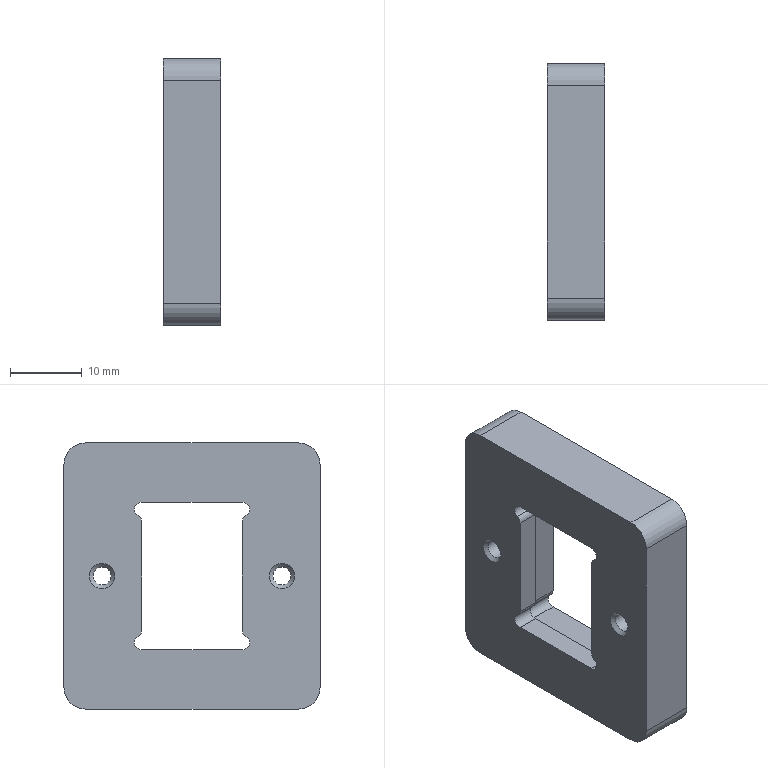Part | 1 solid | 41 faces | box 8 x 35.6 x 37 mm | volume 7524 mm3 | cylinder 22 | plane 15 | cone 4 | commonest cylinder face diameters 2 x16 6 x4 2.5 x2
STEP:
#1=CARTESIAN_POINT('',(288.112,-119.094,41.623));
#2=VERTEX_POINT('',#1);
#3=CARTESIAN_POINT('',(288.112,-122.094,38.623));
#4=VERTEX_POINT('',#3);
#5=CARTESIAN_POINT('',(288.112,-122.094,41.623));
#6=DIRECTION('',(-1.,0.,0.));
#7=DIRECTION('',(0.,-1.,0.));
#8=AXIS2_PLACEMENT_3D('',#5,#6,#7);
#9=CIRCLE('',#8,3.);
#10=EDGE_CURVE('',#2,#4,#9,.T.);
#11=ORIENTED_EDGE('',*,*,#10,.F.);
#12=CARTESIAN_POINT('',(296.112,-119.094,41.623));
#13=VERTEX_POINT('',#12);
#14=CARTESIAN_POINT('',(288.112,-119.094,41.623));
#15=DIRECTION('',(-1.,0.,0.));
#16=VECTOR('',#15,1000.);
#17=LINE('',#14,#16);
#18=EDGE_CURVE('',#13,#2,#17,.T.);
#19=ORIENTED_EDGE('',*,*,#18,.F.);
#20=CARTESIAN_POINT('',(296.112,-122.094,38.623));
#21=VERTEX_POINT('',#20);
#22=CARTESIAN_POINT('',(296.112,-122.094,41.623));
#23=DIRECTION('',(1.,0.,0.));
#24=DIRECTION('',(0.,-1.,0.));
#25=AXIS2_PLACEMENT_3D('',#22,#23,#24);
#26=CIRCLE('',#25,3.);
#27=EDGE_CURVE('',#21,#13,#26,.T.);
#28=ORIENTED_EDGE('',*,*,#27,.F.);
#29=CARTESIAN_POINT('',(288.112,-122.094,38.623));
#30=DIRECTION('',(1.,0.,0.));
#31=VECTOR('',#30,1000.);
#32=LINE('',#29,#31);
#33=EDGE_CURVE('',#4,#21,#32,.T.);
#34=ORIENTED_EDGE('',*,*,#33,.F.);
#35=EDGE_LOOP('',(#11,#19,#28,#34));
#36=FACE_BOUND('',#35,.T.);
#37=CARTESIAN_POINT('',(288.112,-122.094,41.623));
#38=DIRECTION('',(1.,0.,0.));
#39=DIRECTION('',(0.,-1.,0.));
#40=AXIS2_PLACEMENT_3D('',#37,#38,#39);
#41=CYLINDRICAL_SURFACE('',#40,3.);
#42=ADVANCED_FACE('',(#36),#41,.T.);
#43=CARTESIAN_POINT('',(288.112,-122.094,75.623));
#44=VERTEX_POINT('',#43);
#45=CARTESIAN_POINT('',(288.112,-119.094,72.623));
#46=VERTEX_POINT('',#45);
#47=CARTESIAN_POINT('',(288.112,-122.094,72.623));
#48=DIRECTION('',(-1.,0.,0.));
#49=DIRECTION('',(0.,-1.,0.));
#50=AXIS2_PLACEMENT_3D('',#47,#48,#49);
#51=CIRCLE('',#50,3.);
#52=EDGE_CURVE('',#44,#46,#51,.T.);
#53=ORIENTED_EDGE('',*,*,#52,.F.);
#54=CARTESIAN_POINT('',(296.112,-122.094,75.623));
#55=VERTEX_POINT('',#54);
#56=CARTESIAN_POINT('',(288.112,-122.094,75.623));
#57=DIRECTION('',(-1.,0.,0.));
#58=VECTOR('',#57,1000.);
#59=LINE('',#56,#58);
#60=EDGE_CURVE('',#55,#44,#59,.T.);
#61=ORIENTED_EDGE('',*,*,#60,.F.);
#62=CARTESIAN_POINT('',(296.112,-119.094,72.623));
#63=VERTEX_POINT('',#62);
#64=CARTESIAN_POINT('',(296.112,-122.094,72.623));
#65=DIRECTION('',(1.,0.,0.));
#66=DIRECTION('',(0.,-1.,0.));
#67=AXIS2_PLACEMENT_3D('',#64,#65,#66);
#68=CIRCLE('',#67,3.);
#69=EDGE_CURVE('',#63,#55,#68,.T.);
#70=ORIENTED_EDGE('',*,*,#69,.F.);
#71=CARTESIAN_POINT('',(288.112,-119.094,72.623));
#72=DIRECTION('',(1.,0.,0.));
#73=VECTOR('',#72,1000.);
#74=LINE('',#71,#73);
#75=EDGE_CURVE('',#46,#63,#74,.T.);
#76=ORIENTED_EDGE('',*,*,#75,.F.);
#77=EDGE_LOOP('',(#53,#61,#70,#76));
#78=FACE_BOUND('',#77,.T.);
#79=CARTESIAN_POINT('',(288.112,-122.094,72.623));
#80=DIRECTION('',(1.,0.,0.));
#81=DIRECTION('',(0.,-1.,0.));
#82=AXIS2_PLACEMENT_3D('',#79,#80,#81);
#83=CYLINDRICAL_SURFACE('',#82,3.);
#84=ADVANCED_FACE('',(#78),#83,.T.);
#85=CARTESIAN_POINT('',(288.112,-154.694,72.623));
#86=VERTEX_POINT('',#85);
#87=CARTESIAN_POINT('',(288.112,-151.694,75.623));
#88=VERTEX_POINT('',#87);
#89=CARTESIAN_POINT('',(288.112,-151.694,72.623));
#90=DIRECTION('',(-1.,0.,0.));
#91=DIRECTION('',(0.,-1.,0.));
#92=AXIS2_PLACEMENT_3D('',#89,#90,#91);
#93=CIRCLE('',#92,3.);
#94=EDGE_CURVE('',#86,#88,#93,.T.);
#95=ORIENTED_EDGE('',*,*,#94,.F.);
#96=CARTESIAN_POINT('',(296.112,-154.694,72.623));
#97=VERTEX_POINT('',#96);
#98=CARTESIAN_POINT('',(288.112,-154.694,72.623));
#99=DIRECTION('',(-1.,0.,0.));
#100=VECTOR('',#99,1000.);
#101=LINE('',#98,#100);
#102=EDGE_CURVE('',#97,#86,#101,.T.);
#103=ORIENTED_EDGE('',*,*,#102,.F.);
#104=CARTESIAN_POINT('',(296.112,-151.694,75.623));
#105=VERTEX_POINT('',#104);
#106=CARTESIAN_POINT('',(296.112,-151.694,72.623));
#107=DIRECTION('',(1.,0.,0.));
#108=DIRECTION('',(0.,-1.,0.));
#109=AXIS2_PLACEMENT_3D('',#106,#107,#108);
#110=CIRCLE('',#109,3.);
#111=EDGE_CURVE('',#105,#97,#110,.T.);
#112=ORIENTED_EDGE('',*,*,#111,.F.);
#113=CARTESIAN_POINT('',(288.112,-151.694,75.623));
#114=DIRECTION('',(1.,0.,0.));
#115=VECTOR('',#114,1000.);
#116=LINE('',#113,#115);
#117=EDGE_CURVE('',#88,#105,#116,.T.);
#118=ORIENTED_EDGE('',*,*,#117,.F.);
#119=EDGE_LOOP('',(#95,#103,#112,#118));
#120=FACE_BOUND('',#119,.T.);
#121=CARTESIAN_POINT('',(288.112,-151.694,72.623));
#122=DIRECTION('',(1.,0.,0.));
#123=DIRECTION('',(0.,-1.,0.));
#124=AXIS2_PLACEMENT_3D('',#121,#122,#123);
#125=CYLINDRICAL_SURFACE('',#124,3.);
#126=ADVANCED_FACE('',(#120),#125,.T.);
#127=CARTESIAN_POINT('',(288.112,-151.694,38.623));
#128=VERTEX_POINT('',#127);
#129=CARTESIAN_POINT('',(288.112,-154.694,41.623));
#130=VERTEX_POINT('',#129);
#131=CARTESIAN_POINT('',(288.112,-151.694,41.623));
#132=DIRECTION('',(-1.,0.,0.));
#133=DIRECTION('',(0.,-1.,0.));
#134=AXIS2_PLACEMENT_3D('',#131,#132,#133);
#135=CIRCLE('',#134,3.);
#136=EDGE_CURVE('',#128,#130,#135,.T.);
#137=ORIENTED_EDGE('',*,*,#136,.F.);
#138=CARTESIAN_POINT('',(296.112,-151.694,38.623));
#139=VERTEX_POINT('',#138);
#140=CARTESIAN_POINT('',(288.112,-151.694,38.623));
#141=DIRECTION('',(-1.,0.,0.));
#142=VECTOR('',#141,1000.);
#143=LINE('',#140,#142);
#144=EDGE_CURVE('',#139,#128,#143,.T.);
#145=ORIENTED_EDGE('',*,*,#144,.F.);
#146=CARTESIAN_POINT('',(296.112,-154.694,41.623));
#147=VERTEX_POINT('',#146);
#148=CARTESIAN_POINT('',(296.112,-151.694,41.623));
#149=DIRECTION('',(1.,0.,0.));
#150=DIRECTION('',(0.,-1.,0.));
#151=AXIS2_PLACEMENT_3D('',#148,#149,#150);
#152=CIRCLE('',#151,3.);
#153=EDGE_CURVE('',#147,#139,#152,.T.);
#154=ORIENTED_EDGE('',*,*,#153,.F.);
#155=CARTESIAN_POINT('',(288.112,-154.694,41.623));
#156=DIRECTION('',(1.,0.,0.));
#157=VECTOR('',#156,1000.);
#158=LINE('',#155,#157);
#159=EDGE_CURVE('',#130,#147,#158,.T.);
#160=ORIENTED_EDGE('',*,*,#159,.F.);
#161=EDGE_LOOP('',(#137,#145,#154,#160));
#162=FACE_BOUND('',#161,.T.);
#163=CARTESIAN_POINT('',(288.112,-151.694,41.623));
#164=DIRECTION('',(1.,0.,0.));
#165=DIRECTION('',(0.,-1.,0.));
#166=AXIS2_PLACEMENT_3D('',#163,#164,#165);
#167=CYLINDRICAL_SURFACE('',#166,3.);
#168=ADVANCED_FACE('',(#162),#167,.T.);
#169=CARTESIAN_POINT('',(291.112,-127.894,66.757));
#170=VERTEX_POINT('',#169);
#171=CARTESIAN_POINT('',(291.112,-128.394,68.623));
#172=VERTEX_POINT('',#171);
#173=CARTESIAN_POINT('',(291.112,-128.394,67.623));
#174=DIRECTION('',(1.,0.,0.));
#175=DIRECTION('',(0.,-1.,0.));
#176=AXIS2_PLACEMENT_3D('',#173,#174,#175);
#177=CIRCLE('',#176,1.);
#178=EDGE_CURVE('',#170,#172,#177,.T.);
#179=ORIENTED_EDGE('',*,*,#178,.F.);
#180=CARTESIAN_POINT('',(296.112,-127.894,66.757));
#181=VERTEX_POINT('',#180);
#182=CARTESIAN_POINT('',(296.112,-127.894,66.757));
#183=DIRECTION('',(1.,0.,0.));
#184=VECTOR('',#183,1000.);
#185=LINE('',#182,#184);
#186=EDGE_CURVE('',#170,#181,#185,.T.);
#187=ORIENTED_EDGE('',*,*,#186,.T.);
#188=CARTESIAN_POINT('',(296.112,-128.394,68.623));
#189=VERTEX_POINT('',#188);
#190=CARTESIAN_POINT('',(296.112,-128.394,67.623));
#191=DIRECTION('',(1.,0.,0.));
#192=DIRECTION('',(0.,-1.,0.));
#193=AXIS2_PLACEMENT_3D('',#190,#191,#192);
#194=CIRCLE('',#193,1.);
#195=EDGE_CURVE('',#181,#189,#194,.T.);
#196=ORIENTED_EDGE('',*,*,#195,.T.);
#197=CARTESIAN_POINT('',(291.112,-128.394,68.623));
#198=DIRECTION('',(1.,0.,0.));
#199=VECTOR('',#198,1000.);
#200=LINE('',#197,#199);
#201=EDGE_CURVE('',#172,#189,#200,.T.);
#202=ORIENTED_EDGE('',*,*,#201,.F.);
#203=EDGE_LOOP('',(#179,#187,#196,#202));
#204=FACE_BOUND('',#203,.T.);
#205=CARTESIAN_POINT('',(296.112,-128.394,67.623));
#206=DIRECTION('',(1.,0.,0.));
#207=DIRECTION('',(0.,-1.,0.));
#208=AXIS2_PLACEMENT_3D('',#205,#206,#207);
#209=CYLINDRICAL_SURFACE('',#208,1.);
#210=ADVANCED_FACE('',(#204),#209,.F.);
#211=CARTESIAN_POINT('',(296.112,-128.394,45.623));
#212=VERTEX_POINT('',#211);
#213=CARTESIAN_POINT('',(296.112,-127.894,47.489));
#214=VERTEX_POINT('',#213);
#215=CARTESIAN_POINT('',(296.112,-128.394,46.623));
#216=DIRECTION('',(1.,0.,0.));
#217=DIRECTION('',(0.,-1.,0.));
#218=AXIS2_PLACEMENT_3D('',#215,#216,#217);
#219=CIRCLE('',#218,1.);
#220=EDGE_CURVE('',#212,#214,#219,.T.);
#221=ORIENTED_EDGE('',*,*,#220,.T.);
#222=CARTESIAN_POINT('',(291.112,-127.894,47.489));
#223=VERTEX_POINT('',#222);
#224=CARTESIAN_POINT('',(296.112,-127.894,47.489));
#225=DIRECTION('',(1.,0.,0.));
#226=VECTOR('',#225,1000.);
#227=LINE('',#224,#226);
#228=EDGE_CURVE('',#214,#223,#227,.F.);
#229=ORIENTED_EDGE('',*,*,#228,.T.);
#230=CARTESIAN_POINT('',(291.112,-128.394,45.623));
#231=VERTEX_POINT('',#230);
#232=CARTESIAN_POINT('',(291.112,-128.394,46.623));
#233=DIRECTION('',(1.,0.,0.));
#234=DIRECTION('',(0.,-1.,0.));
#235=AXIS2_PLACEMENT_3D('',#232,#233,#234);
#236=CIRCLE('',#235,1.);
#237=EDGE_CURVE('',#231,#223,#236,.T.);
#238=ORIENTED_EDGE('',*,*,#237,.F.);
#239=CARTESIAN_POINT('',(291.112,-128.394,45.623));
#240=DIRECTION('',(1.,0.,0.));
#241=VECTOR('',#240,1000.);
#242=LINE('',#239,#241);
#243=EDGE_CURVE('',#231,#212,#242,.T.);
#244=ORIENTED_EDGE('',*,*,#243,.T.);
#245=EDGE_LOOP('',(#221,#229,#238,#244));
#246=FACE_BOUND('',#245,.T.);
#247=CARTESIAN_POINT('',(296.112,-128.394,46.623));
#248=DIRECTION('',(1.,0.,0.));
#249=DIRECTION('',(0.,-1.,0.));
#250=AXIS2_PLACEMENT_3D('',#247,#248,#249);
#251=CYLINDRICAL_SURFACE('',#250,1.);
#252=ADVANCED_FACE('',(#246),#251,.F.);
#253=CARTESIAN_POINT('',(288.112,-129.394,65.507));
#254=VERTEX_POINT('',#253);
#255=CARTESIAN_POINT('',(288.112,-129.894,67.373));
#256=VERTEX_POINT('',#255);
#257=CARTESIAN_POINT('',(288.112,-129.894,66.373));
#258=DIRECTION('',(1.,0.,0.));
#259=DIRECTION('',(0.,-1.,0.));
#260=AXIS2_PLACEMENT_3D('',#257,#258,#259);
#261=CIRCLE('',#260,1.);
#262=EDGE_CURVE('',#254,#256,#261,.T.);
#263=ORIENTED_EDGE('',*,*,#262,.F.);
#264=CARTESIAN_POINT('',(291.112,-129.394,65.507));
#265=VERTEX_POINT('',#264);
#266=CARTESIAN_POINT('',(288.112,-129.394,65.507));
#267=DIRECTION('',(1.,0.,0.));
#268=VECTOR('',#267,1000.);
#269=LINE('',#266,#268);
#270=EDGE_CURVE('',#254,#265,#269,.T.);
#271=ORIENTED_EDGE('',*,*,#270,.T.);
#272=CARTESIAN_POINT('',(291.112,-129.894,67.373));
#273=VERTEX_POINT('',#272);
#274=CARTESIAN_POINT('',(291.112,-129.894,66.373));
#275=DIRECTION('',(1.,0.,0.));
#276=DIRECTION('',(0.,-1.,0.));
#277=AXIS2_PLACEMENT_3D('',#274,#275,#276);
#278=CIRCLE('',#277,1.);
#279=EDGE_CURVE('',#265,#273,#278,.T.);
#280=ORIENTED_EDGE('',*,*,#279,.T.);
#281=CARTESIAN_POINT('',(288.112,-129.894,67.373));
#282=DIRECTION('',(1.,0.,0.));
#283=VECTOR('',#282,1000.);
#284=LINE('',#281,#283);
#285=EDGE_CURVE('',#256,#273,#284,.T.);
#286=ORIENTED_EDGE('',*,*,#285,.F.);
#287=EDGE_LOOP('',(#263,#271,#280,#286));
#288=FACE_BOUND('',#287,.T.);
#289=CARTESIAN_POINT('',(288.112,-129.894,66.373));
#290=DIRECTION('',(1.,0.,0.));
#291=DIRECTION('',(0.,-1.,0.));
#292=AXIS2_PLACEMENT_3D('',#289,#290,#291);
#293=CYLINDRICAL_SURFACE('',#292,1.);
#294=ADVANCED_FACE('',(#288),#293,.F.);
#295=CARTESIAN_POINT('',(291.112,-129.894,46.873));
#296=VERTEX_POINT('',#295);
#297=CARTESIAN_POINT('',(291.112,-129.394,48.739));
#298=VERTEX_POINT('',#297);
#299=CARTESIAN_POINT('',(291.112,-129.894,47.873));
#300=DIRECTION('',(1.,0.,0.));
#301=DIRECTION('',(0.,-1.,0.));
#302=AXIS2_PLACEMENT_3D('',#299,#300,#301);
#303=CIRCLE('',#302,1.);
#304=EDGE_CURVE('',#296,#298,#303,.T.);
#305=ORIENTED_EDGE('',*,*,#304,.T.);
#306=CARTESIAN_POINT('',(288.112,-129.394,48.739));
#307=VERTEX_POINT('',#306);
#308=CARTESIAN_POINT('',(288.112,-129.394,48.739));
#309=DIRECTION('',(1.,0.,0.));
#310=VECTOR('',#309,1000.);
#311=LINE('',#308,#310);
#312=EDGE_CURVE('',#298,#307,#311,.F.);
#313=ORIENTED_EDGE('',*,*,#312,.T.);
#314=CARTESIAN_POINT('',(288.112,-129.894,46.873));
#315=VERTEX_POINT('',#314);
#316=CARTESIAN_POINT('',(288.112,-129.894,47.873));
#317=DIRECTION('',(1.,0.,0.));
#318=DIRECTION('',(0.,-1.,0.));
#319=AXIS2_PLACEMENT_3D('',#316,#317,#318);
#320=CIRCLE('',#319,1.);
#321=EDGE_CURVE('',#315,#307,#320,.T.);
#322=ORIENTED_EDGE('',*,*,#321,.F.);
#323=CARTESIAN_POINT('',(288.112,-129.894,46.873));
#324=DIRECTION('',(1.,0.,0.));
#325=VECTOR('',#324,1000.);
#326=LINE('',#323,#325);
#327=EDGE_CURVE('',#315,#296,#326,.T.);
#328=ORIENTED_EDGE('',*,*,#327,.T.);
#329=EDGE_LOOP('',(#305,#313,#322,#328));
#330=FACE_BOUND('',#329,.T.);
#331=CARTESIAN_POINT('',(288.112,-129.894,47.873));
#332=DIRECTION('',(1.,0.,0.));
#333=DIRECTION('',(0.,-1.,0.));
#334=AXIS2_PLACEMENT_3D('',#331,#332,#333);
#335=CYLINDRICAL_SURFACE('',#334,1.);
#336=ADVANCED_FACE('',(#330),#335,.F.);
#337=CARTESIAN_POINT('',(296.112,-145.394,45.623));
#338=VERTEX_POINT('',#337);
#339=CARTESIAN_POINT('',(296.112,-128.394,45.623));
#340=DIRECTION('',(0.,1.,0.));
#341=VECTOR('',#340,1000.);
#342=LINE('',#339,#341);
#343=EDGE_CURVE('',#338,#212,#342,.T.);
#344=ORIENTED_EDGE('',*,*,#343,.T.);
#345=ORIENTED_EDGE('',*,*,#243,.F.);
#346=CARTESIAN_POINT('',(291.112,-145.394,45.623));
#347=VERTEX_POINT('',#346);
#348=CARTESIAN_POINT('',(291.112,-128.394,45.623));
#349=DIRECTION('',(0.,1.,0.));
#350=VECTOR('',#349,1000.);
#351=LINE('',#348,#350);
#352=EDGE_CURVE('',#347,#231,#351,.T.);
#353=ORIENTED_EDGE('',*,*,#352,.F.);
#354=CARTESIAN_POINT('',(291.112,-145.394,45.623));
#355=DIRECTION('',(1.,0.,0.));
#356=VECTOR('',#355,1000.);
#357=LINE('',#354,#356);
#358=EDGE_CURVE('',#347,#338,#357,.T.);
#359=ORIENTED_EDGE('',*,*,#358,.T.);
#360=EDGE_LOOP('',(#344,#345,#353,#359));
#361=FACE_BOUND('',#360,.T.);
#362=CARTESIAN_POINT('',(291.112,-128.394,45.623));
#363=DIRECTION('',(0.,0.,-1.));
#364=DIRECTION('',(-1.,0.,0.));
#365=AXIS2_PLACEMENT_3D('',#362,#363,#364);
#366=PLANE('',#365);
#367=ADVANCED_FACE('',(#361),#366,.F.);
#368=CARTESIAN_POINT('',(296.112,-145.394,68.623));
#369=VERTEX_POINT('',#368);
#370=CARTESIAN_POINT('',(296.112,-128.394,68.623));
#371=DIRECTION('',(0.,-1.,0.));
#372=VECTOR('',#371,1000.);
#373=LINE('',#370,#372);
#374=EDGE_CURVE('',#189,#369,#373,.T.);
#375=ORIENTED_EDGE('',*,*,#374,.T.);
#376=CARTESIAN_POINT('',(291.112,-145.394,68.623));
#377=VERTEX_POINT('',#376);
#378=CARTESIAN_POINT('',(291.112,-145.394,68.623));
#379=DIRECTION('',(1.,0.,0.));
#380=VECTOR('',#379,1000.);
#381=LINE('',#378,#380);
#382=EDGE_CURVE('',#377,#369,#381,.T.);
#383=ORIENTED_EDGE('',*,*,#382,.F.);
#384=CARTESIAN_POINT('',(291.112,-128.394,68.623));
#385=DIRECTION('',(0.,-1.,0.));
#386=VECTOR('',#385,1000.);
#387=LINE('',#384,#386);
#388=EDGE_CURVE('',#172,#377,#387,.T.);
#389=ORIENTED_EDGE('',*,*,#388,.F.);
#390=ORIENTED_EDGE('',*,*,#201,.T.);
#391=EDGE_LOOP('',(#375,#383,#389,#390));
#392=FACE_BOUND('',#391,.T.);
#393=CARTESIAN_POINT('',(291.112,-128.394,68.623));
#394=DIRECTION('',(0.,0.,1.));
#395=DIRECTION('',(0.,-1.,0.));
#396=AXIS2_PLACEMENT_3D('',#393,#394,#395);
#397=PLANE('',#396);
#398=ADVANCED_FACE('',(#392),#397,.F.);
#399=ORIENTED_EDGE('',*,*,#388,.T.);
#400=CARTESIAN_POINT('',(291.112,-145.894,66.757));
#401=VERTEX_POINT('',#400);
#402=CARTESIAN_POINT('',(291.112,-145.394,67.623));
#403=DIRECTION('',(1.,0.,0.));
#404=DIRECTION('',(0.,-1.,0.));
#405=AXIS2_PLACEMENT_3D('',#402,#403,#404);
#406=CIRCLE('',#405,1.);
#407=EDGE_CURVE('',#377,#401,#406,.T.);
#408=ORIENTED_EDGE('',*,*,#407,.T.);
#409=CARTESIAN_POINT('',(291.112,-145.394,65.891));
#410=VERTEX_POINT('',#409);
#411=CARTESIAN_POINT('',(291.112,-146.394,65.891));
#412=DIRECTION('',(1.,0.,0.));
#413=DIRECTION('',(0.,0.,-1.));
#414=AXIS2_PLACEMENT_3D('',#411,#412,#413);
#415=CIRCLE('',#414,1.);
#416=EDGE_CURVE('',#401,#410,#415,.F.);
#417=ORIENTED_EDGE('',*,*,#416,.T.);
#418=CARTESIAN_POINT('',(291.112,-145.394,48.355));
#419=VERTEX_POINT('',#418);
#420=CARTESIAN_POINT('',(291.112,-145.394,45.623));
#421=DIRECTION('',(0.,0.,-1.));
#422=VECTOR('',#421,1000.);
#423=LINE('',#420,#422);
#424=EDGE_CURVE('',#410,#419,#423,.T.);
#425=ORIENTED_EDGE('',*,*,#424,.T.);
#426=CARTESIAN_POINT('',(291.112,-145.894,47.489));
#427=VERTEX_POINT('',#426);
#428=CARTESIAN_POINT('',(291.112,-146.394,48.355));
#429=DIRECTION('',(1.,0.,0.));
#430=DIRECTION('',(0.,0.,-1.));
#431=AXIS2_PLACEMENT_3D('',#428,#429,#430);
#432=CIRCLE('',#431,1.);
#433=EDGE_CURVE('',#419,#427,#432,.F.);
#434=ORIENTED_EDGE('',*,*,#433,.T.);
#435=CARTESIAN_POINT('',(291.112,-145.394,46.623));
#436=DIRECTION('',(1.,0.,0.));
#437=DIRECTION('',(0.,-1.,0.));
#438=AXIS2_PLACEMENT_3D('',#435,#436,#437);
#439=CIRCLE('',#438,1.);
#440=EDGE_CURVE('',#427,#347,#439,.T.);
#441=ORIENTED_EDGE('',*,*,#440,.T.);
#442=ORIENTED_EDGE('',*,*,#352,.T.);
#443=ORIENTED_EDGE('',*,*,#237,.T.);
#444=CARTESIAN_POINT('',(291.112,-128.394,48.355));
#445=VERTEX_POINT('',#444);
#446=CARTESIAN_POINT('',(291.112,-127.394,48.355));
#447=DIRECTION('',(1.,0.,0.));
#448=DIRECTION('',(0.,0.,-1.));
#449=AXIS2_PLACEMENT_3D('',#446,#447,#448);
#450=CIRCLE('',#449,1.);
#451=EDGE_CURVE('',#223,#445,#450,.F.);
#452=ORIENTED_EDGE('',*,*,#451,.T.);
#453=CARTESIAN_POINT('',(291.112,-128.394,65.891));
#454=VERTEX_POINT('',#453);
#455=CARTESIAN_POINT('',(291.112,-128.394,45.623));
#456=DIRECTION('',(0.,0.,1.));
#457=VECTOR('',#456,1000.);
#458=LINE('',#455,#457);
#459=EDGE_CURVE('',#445,#454,#458,.T.);
#460=ORIENTED_EDGE('',*,*,#459,.T.);
#461=CARTESIAN_POINT('',(291.112,-127.394,65.891));
#462=DIRECTION('',(1.,0.,0.));
#463=DIRECTION('',(0.,0.,-1.));
#464=AXIS2_PLACEMENT_3D('',#461,#462,#463);
#465=CIRCLE('',#464,1.);
#466=EDGE_CURVE('',#454,#170,#465,.F.);
#467=ORIENTED_EDGE('',*,*,#466,.T.);
#468=ORIENTED_EDGE('',*,*,#178,.T.);
#469=EDGE_LOOP('',(#399,#408,#417,#425,#434,#441,#442,#443,#452,#460,#467,#468));
#470=FACE_BOUND('',#469,.T.);
#471=CARTESIAN_POINT('',(291.112,-129.894,64.641));
#472=VERTEX_POINT('',#471);
#473=CARTESIAN_POINT('',(291.112,-129.894,49.605));
#474=VERTEX_POINT('',#473);
#475=CARTESIAN_POINT('',(291.112,-129.894,46.873));
#476=DIRECTION('',(0.,0.,-1.));
#477=VECTOR('',#476,1000.);
#478=LINE('',#475,#477);
#479=EDGE_CURVE('',#472,#474,#478,.T.);
#480=ORIENTED_EDGE('',*,*,#479,.T.);
#481=CARTESIAN_POINT('',(291.112,-128.894,49.605));
#482=DIRECTION('',(1.,0.,0.));
#483=DIRECTION('',(0.,0.,-1.));
#484=AXIS2_PLACEMENT_3D('',#481,#482,#483);
#485=CIRCLE('',#484,1.);
#486=EDGE_CURVE('',#474,#298,#485,.T.);
#487=ORIENTED_EDGE('',*,*,#486,.T.);
#488=ORIENTED_EDGE('',*,*,#304,.F.);
#489=CARTESIAN_POINT('',(291.112,-143.894,46.873));
#490=VERTEX_POINT('',#489);
#491=CARTESIAN_POINT('',(291.112,-129.894,46.873));
#492=DIRECTION('',(0.,-1.,0.));
#493=VECTOR('',#492,1000.);
#494=LINE('',#491,#493);
#495=EDGE_CURVE('',#296,#490,#494,.T.);
#496=ORIENTED_EDGE('',*,*,#495,.T.);
#497=CARTESIAN_POINT('',(291.112,-144.394,48.739));
#498=VERTEX_POINT('',#497);
#499=CARTESIAN_POINT('',(291.112,-143.894,47.873));
#500=DIRECTION('',(1.,0.,0.));
#501=DIRECTION('',(0.,-1.,0.));
#502=AXIS2_PLACEMENT_3D('',#499,#500,#501);
#503=CIRCLE('',#502,1.);
#504=EDGE_CURVE('',#498,#490,#503,.T.);
#505=ORIENTED_EDGE('',*,*,#504,.F.);
#506=CARTESIAN_POINT('',(291.112,-143.894,49.605));
#507=VERTEX_POINT('',#506);
#508=CARTESIAN_POINT('',(291.112,-144.894,49.605));
#509=DIRECTION('',(1.,0.,0.));
#510=DIRECTION('',(0.,0.,-1.));
#511=AXIS2_PLACEMENT_3D('',#508,#509,#510);
#512=CIRCLE('',#511,1.);
#513=EDGE_CURVE('',#498,#507,#512,.T.);
#514=ORIENTED_EDGE('',*,*,#513,.T.);
#515=CARTESIAN_POINT('',(291.112,-143.894,64.641));
#516=VERTEX_POINT('',#515);
#517=CARTESIAN_POINT('',(291.112,-143.894,46.873));
#518=DIRECTION('',(0.,0.,1.));
#519=VECTOR('',#518,1000.);
#520=LINE('',#517,#519);
#521=EDGE_CURVE('',#507,#516,#520,.T.);
#522=ORIENTED_EDGE('',*,*,#521,.T.);
#523=CARTESIAN_POINT('',(291.112,-144.394,65.507));
#524=VERTEX_POINT('',#523);
#525=CARTESIAN_POINT('',(291.112,-144.894,64.641));
#526=DIRECTION('',(1.,0.,0.));
#527=DIRECTION('',(0.,0.,-1.));
#528=AXIS2_PLACEMENT_3D('',#525,#526,#527);
#529=CIRCLE('',#528,1.);
#530=EDGE_CURVE('',#516,#524,#529,.T.);
#531=ORIENTED_EDGE('',*,*,#530,.T.);
#532=CARTESIAN_POINT('',(291.112,-143.894,67.373));
#533=VERTEX_POINT('',#532);
#534=CARTESIAN_POINT('',(291.112,-143.894,66.373));
#535=DIRECTION('',(1.,0.,0.));
#536=DIRECTION('',(0.,-1.,0.));
#537=AXIS2_PLACEMENT_3D('',#534,#535,#536);
#538=CIRCLE('',#537,1.);
#539=EDGE_CURVE('',#533,#524,#538,.T.);
#540=ORIENTED_EDGE('',*,*,#539,.F.);
#541=CARTESIAN_POINT('',(291.112,-129.894,67.373));
#542=DIRECTION('',(0.,1.,0.));
#543=VECTOR('',#542,1000.);
#544=LINE('',#541,#543);
#545=EDGE_CURVE('',#533,#273,#544,.T.);
#546=ORIENTED_EDGE('',*,*,#545,.T.);
#547=ORIENTED_EDGE('',*,*,#279,.F.);
#548=CARTESIAN_POINT('',(291.112,-128.894,64.641));
#549=DIRECTION('',(1.,0.,0.));
#550=DIRECTION('',(0.,0.,-1.));
#551=AXIS2_PLACEMENT_3D('',#548,#549,#550);
#552=CIRCLE('',#551,1.);
#553=EDGE_CURVE('',#265,#472,#552,.T.);
#554=ORIENTED_EDGE('',*,*,#553,.T.);
#555=EDGE_LOOP('',(#480,#487,#488,#496,#505,#514,#522,#531,#540,#546,#547,#554));
#556=FACE_BOUND('',#555,.T.);
#557=CARTESIAN_POINT('',(291.112,-136.894,57.123));
#558=DIRECTION('',(1.,0.,0.));
#559=DIRECTION('',(0.,0.,1.));
#560=AXIS2_PLACEMENT_3D('',#557,#558,#559);
#561=PLANE('',#560);
#562=ADVANCED_FACE('',(#470,#556),#561,.T.);
#563=CARTESIAN_POINT('',(296.112,-154.694,38.623));
#564=DIRECTION('',(0.,0.,-1.));
#565=VECTOR('',#564,1000.);
#566=LINE('',#563,#565);
#567=EDGE_CURVE('',#97,#147,#566,.T.);
#568=ORIENTED_EDGE('',*,*,#567,.T.);
#569=ORIENTED_EDGE('',*,*,#153,.T.);
#570=CARTESIAN_POINT('',(296.112,-119.094,38.623));
#571=DIRECTION('',(0.,1.,0.));
#572=VECTOR('',#571,1000.);
#573=LINE('',#570,#572);
#574=EDGE_CURVE('',#139,#21,#573,.T.);
#575=ORIENTED_EDGE('',*,*,#574,.T.);
#576=ORIENTED_EDGE('',*,*,#27,.T.);
#577=CARTESIAN_POINT('',(296.112,-119.094,38.623));
#578=DIRECTION('',(0.,0.,1.));
#579=VECTOR('',#578,1000.);
#580=LINE('',#577,#579);
#581=EDGE_CURVE('',#13,#63,#580,.T.);
#582=ORIENTED_EDGE('',*,*,#581,.T.);
#583=ORIENTED_EDGE('',*,*,#69,.T.);
#584=CARTESIAN_POINT('',(296.112,-119.094,75.623));
#585=DIRECTION('',(0.,-1.,0.));
#586=VECTOR('',#585,1000.);
#587=LINE('',#584,#586);
#588=EDGE_CURVE('',#55,#105,#587,.T.);
#589=ORIENTED_EDGE('',*,*,#588,.T.);
#590=ORIENTED_EDGE('',*,*,#111,.T.);
#591=EDGE_LOOP('',(#568,#569,#575,#576,#582,#583,#589,#590));
#592=FACE_BOUND('',#591,.T.);
#593=CARTESIAN_POINT('',(296.112,-128.394,48.355));
#594=VERTEX_POINT('',#593);
#595=CARTESIAN_POINT('',(296.112,-128.394,65.891));
#596=VERTEX_POINT('',#595);
#597=CARTESIAN_POINT('',(296.112,-128.394,45.623));
#598=DIRECTION('',(0.,0.,1.));
#599=VECTOR('',#598,1000.);
#600=LINE('',#597,#599);
#601=EDGE_CURVE('',#594,#596,#600,.T.);
#602=ORIENTED_EDGE('',*,*,#601,.F.);
#603=CARTESIAN_POINT('',(296.112,-127.394,48.355));
#604=DIRECTION('',(1.,0.,0.));
#605=DIRECTION('',(0.,0.,-1.));
#606=AXIS2_PLACEMENT_3D('',#603,#604,#605);
#607=CIRCLE('',#606,1.);
#608=EDGE_CURVE('',#594,#214,#607,.T.);
#609=ORIENTED_EDGE('',*,*,#608,.T.);
#610=ORIENTED_EDGE('',*,*,#220,.F.);
#611=ORIENTED_EDGE('',*,*,#343,.F.);
#612=CARTESIAN_POINT('',(296.112,-145.894,47.489));
#613=VERTEX_POINT('',#612);
#614=CARTESIAN_POINT('',(296.112,-145.394,46.623));
#615=DIRECTION('',(1.,0.,0.));
#616=DIRECTION('',(0.,-1.,0.));
#617=AXIS2_PLACEMENT_3D('',#614,#615,#616);
#618=CIRCLE('',#617,1.);
#619=EDGE_CURVE('',#613,#338,#618,.T.);
#620=ORIENTED_EDGE('',*,*,#619,.F.);
#621=CARTESIAN_POINT('',(296.112,-145.394,48.355));
#622=VERTEX_POINT('',#621);
#623=CARTESIAN_POINT('',(296.112,-146.394,48.355));
#624=DIRECTION('',(1.,0.,0.));
#625=DIRECTION('',(0.,0.,-1.));
#626=AXIS2_PLACEMENT_3D('',#623,#624,#625);
#627=CIRCLE('',#626,1.);
#628=EDGE_CURVE('',#613,#622,#627,.T.);
#629=ORIENTED_EDGE('',*,*,#628,.T.);
#630=CARTESIAN_POINT('',(296.112,-145.394,65.891));
#631=VERTEX_POINT('',#630);
#632=CARTESIAN_POINT('',(296.112,-145.394,45.623));
#633=DIRECTION('',(0.,0.,-1.));
#634=VECTOR('',#633,1000.);
#635=LINE('',#632,#634);
#636=EDGE_CURVE('',#631,#622,#635,.T.);
#637=ORIENTED_EDGE('',*,*,#636,.F.);
#638=CARTESIAN_POINT('',(296.112,-145.894,66.757));
#639=VERTEX_POINT('',#638);
#640=CARTESIAN_POINT('',(296.112,-146.394,65.891));
#641=DIRECTION('',(1.,0.,0.));
#642=DIRECTION('',(0.,0.,-1.));
#643=AXIS2_PLACEMENT_3D('',#640,#641,#642);
#644=CIRCLE('',#643,1.);
#645=EDGE_CURVE('',#631,#639,#644,.T.);
#646=ORIENTED_EDGE('',*,*,#645,.T.);
#647=CARTESIAN_POINT('',(296.112,-145.394,67.623));
#648=DIRECTION('',(1.,0.,0.));
#649=DIRECTION('',(0.,-1.,0.));
#650=AXIS2_PLACEMENT_3D('',#647,#648,#649);
#651=CIRCLE('',#650,1.);
#652=EDGE_CURVE('',#369,#639,#651,.T.);
#653=ORIENTED_EDGE('',*,*,#652,.F.);
#654=ORIENTED_EDGE('',*,*,#374,.F.);
#655=ORIENTED_EDGE('',*,*,#195,.F.);
#656=CARTESIAN_POINT('',(296.112,-127.394,65.891));
#657=DIRECTION('',(1.,0.,0.));
#658=DIRECTION('',(0.,0.,-1.));
#659=AXIS2_PLACEMENT_3D('',#656,#657,#658);
#660=CIRCLE('',#659,1.);
#661=EDGE_CURVE('',#181,#596,#660,.T.);
#662=ORIENTED_EDGE('',*,*,#661,.T.);
#663=EDGE_LOOP('',(#602,#609,#610,#611,#620,#629,#637,#646,#653,#654,#655,#662));
#664=FACE_BOUND('',#663,.T.);
#665=CARTESIAN_POINT('',(296.112,-126.144,57.123));
#666=VERTEX_POINT('',#665);
#667=CARTESIAN_POINT('',(296.112,-124.394,57.123));
#668=DIRECTION('',(-1.,0.,0.));
#669=DIRECTION('',(0.,-1.,0.));
#670=AXIS2_PLACEMENT_3D('',#667,#668,#669);
#671=CIRCLE('',#670,1.75);
#672=EDGE_CURVE('',#666,#666,#671,.T.);
#673=ORIENTED_EDGE('',*,*,#672,.T.);
#674=EDGE_LOOP('',(#673));
#675=FACE_BOUND('',#674,.T.);
#676=CARTESIAN_POINT('',(296.112,-151.144,57.123));
#677=VERTEX_POINT('',#676);
#678=CARTESIAN_POINT('',(296.112,-149.394,57.123));
#679=DIRECTION('',(-1.,0.,0.));
#680=DIRECTION('',(0.,-1.,0.));
#681=AXIS2_PLACEMENT_3D('',#678,#679,#680);
#682=CIRCLE('',#681,1.75);
#683=EDGE_CURVE('',#677,#677,#682,.T.);
#684=ORIENTED_EDGE('',*,*,#683,.T.);
#685=EDGE_LOOP('',(#684));
#686=FACE_BOUND('',#685,.T.);
#687=CARTESIAN_POINT('',(296.112,-136.894,57.123));
#688=DIRECTION('',(1.,0.,0.));
#689=DIRECTION('',(0.,0.,1.));
#690=AXIS2_PLACEMENT_3D('',#687,#688,#689);
#691=PLANE('',#690);
#692=ADVANCED_FACE('',(#592,#664,#675,#686),#691,.T.);
#693=CARTESIAN_POINT('',(288.112,-119.094,38.623));
#694=DIRECTION('',(0.,1.,0.));
#695=VECTOR('',#694,1000.);
#696=LINE('',#693,#695);
#697=EDGE_CURVE('',#128,#4,#696,.T.);
#698=ORIENTED_EDGE('',*,*,#697,.F.);
#699=ORIENTED_EDGE('',*,*,#136,.T.);
#700=CARTESIAN_POINT('',(288.112,-154.694,38.623));
#701=DIRECTION('',(0.,0.,-1.));
#702=VECTOR('',#701,1000.);
#703=LINE('',#700,#702);
#704=EDGE_CURVE('',#86,#130,#703,.T.);
#705=ORIENTED_EDGE('',*,*,#704,.F.);
#706=ORIENTED_EDGE('',*,*,#94,.T.);
#707=CARTESIAN_POINT('',(288.112,-119.094,75.623));
#708=DIRECTION('',(0.,-1.,0.));
#709=VECTOR('',#708,1000.);
#710=LINE('',#707,#709);
#711=EDGE_CURVE('',#44,#88,#710,.T.);
#712=ORIENTED_EDGE('',*,*,#711,.F.);
#713=ORIENTED_EDGE('',*,*,#52,.T.);
#714=CARTESIAN_POINT('',(288.112,-119.094,38.623));
#715=DIRECTION('',(0.,0.,1.));
#716=VECTOR('',#715,1000.);
#717=LINE('',#714,#716);
#718=EDGE_CURVE('',#2,#46,#717,.T.);
#719=ORIENTED_EDGE('',*,*,#718,.F.);
#720=ORIENTED_EDGE('',*,*,#10,.T.);
#721=EDGE_LOOP('',(#698,#699,#705,#706,#712,#713,#719,#720));
#722=FACE_BOUND('',#721,.T.);
#723=ORIENTED_EDGE('',*,*,#321,.T.);
#724=CARTESIAN_POINT('',(288.112,-129.894,49.605));
#725=VERTEX_POINT('',#724);
#726=CARTESIAN_POINT('',(288.112,-128.894,49.605));
#727=DIRECTION('',(1.,0.,0.));
#728=DIRECTION('',(0.,0.,-1.));
#729=AXIS2_PLACEMENT_3D('',#726,#727,#728);
#730=CIRCLE('',#729,1.);
#731=EDGE_CURVE('',#307,#725,#730,.F.);
#732=ORIENTED_EDGE('',*,*,#731,.T.);
#733=CARTESIAN_POINT('',(288.112,-129.894,64.641));
#734=VERTEX_POINT('',#733);
#735=CARTESIAN_POINT('',(288.112,-129.894,46.873));
#736=DIRECTION('',(0.,0.,1.));
#737=VECTOR('',#736,1000.);
#738=LINE('',#735,#737);
#739=EDGE_CURVE('',#725,#734,#738,.T.);
#740=ORIENTED_EDGE('',*,*,#739,.T.);
#741=CARTESIAN_POINT('',(288.112,-128.894,64.641));
#742=DIRECTION('',(1.,0.,0.));
#743=DIRECTION('',(0.,0.,-1.));
#744=AXIS2_PLACEMENT_3D('',#741,#742,#743);
#745=CIRCLE('',#744,1.);
#746=EDGE_CURVE('',#734,#254,#745,.F.);
#747=ORIENTED_EDGE('',*,*,#746,.T.);
#748=ORIENTED_EDGE('',*,*,#262,.T.);
#749=CARTESIAN_POINT('',(288.112,-143.894,67.373));
#750=VERTEX_POINT('',#749);
#751=CARTESIAN_POINT('',(288.112,-129.894,67.373));
#752=DIRECTION('',(0.,-1.,0.));
#753=VECTOR('',#752,1000.);
#754=LINE('',#751,#753);
#755=EDGE_CURVE('',#256,#750,#754,.T.);
#756=ORIENTED_EDGE('',*,*,#755,.T.);
#757=CARTESIAN_POINT('',(288.112,-144.394,65.507));
#758=VERTEX_POINT('',#757);
#759=CARTESIAN_POINT('',(288.112,-143.894,66.373));
#760=DIRECTION('',(1.,0.,0.));
#761=DIRECTION('',(0.,-1.,0.));
#762=AXIS2_PLACEMENT_3D('',#759,#760,#761);
#763=CIRCLE('',#762,1.);
#764=EDGE_CURVE('',#750,#758,#763,.T.);
#765=ORIENTED_EDGE('',*,*,#764,.T.);
#766=CARTESIAN_POINT('',(288.112,-143.894,64.641));
#767=VERTEX_POINT('',#766);
#768=CARTESIAN_POINT('',(288.112,-144.894,64.641));
#769=DIRECTION('',(1.,0.,0.));
#770=DIRECTION('',(0.,0.,-1.));
#771=AXIS2_PLACEMENT_3D('',#768,#769,#770);
#772=CIRCLE('',#771,1.);
#773=EDGE_CURVE('',#758,#767,#772,.F.);
#774=ORIENTED_EDGE('',*,*,#773,.T.);
#775=CARTESIAN_POINT('',(288.112,-143.894,49.605));
#776=VERTEX_POINT('',#775);
#777=CARTESIAN_POINT('',(288.112,-143.894,46.873));
#778=DIRECTION('',(0.,0.,-1.));
#779=VECTOR('',#778,1000.);
#780=LINE('',#777,#779);
#781=EDGE_CURVE('',#767,#776,#780,.T.);
#782=ORIENTED_EDGE('',*,*,#781,.T.);
#783=CARTESIAN_POINT('',(288.112,-144.394,48.739));
#784=VERTEX_POINT('',#783);
#785=CARTESIAN_POINT('',(288.112,-144.894,49.605));
#786=DIRECTION('',(1.,0.,0.));
#787=DIRECTION('',(0.,0.,-1.));
#788=AXIS2_PLACEMENT_3D('',#785,#786,#787);
#789=CIRCLE('',#788,1.);
#790=EDGE_CURVE('',#776,#784,#789,.F.);
#791=ORIENTED_EDGE('',*,*,#790,.T.);
#792=CARTESIAN_POINT('',(288.112,-143.894,46.873));
#793=VERTEX_POINT('',#792);
#794=CARTESIAN_POINT('',(288.112,-143.894,47.873));
#795=DIRECTION('',(1.,0.,0.));
#796=DIRECTION('',(0.,-1.,0.));
#797=AXIS2_PLACEMENT_3D('',#794,#795,#796);
#798=CIRCLE('',#797,1.);
#799=EDGE_CURVE('',#784,#793,#798,.T.);
#800=ORIENTED_EDGE('',*,*,#799,.T.);
#801=CARTESIAN_POINT('',(288.112,-129.894,46.873));
#802=DIRECTION('',(0.,1.,0.));
#803=VECTOR('',#802,1000.);
#804=LINE('',#801,#803);
#805=EDGE_CURVE('',#793,#315,#804,.T.);
#806=ORIENTED_EDGE('',*,*,#805,.T.);
#807=EDGE_LOOP('',(#723,#732,#740,#747,#748,#756,#765,#774,#782,#791,#800,#806));
#808=FACE_BOUND('',#807,.T.);
#809=CARTESIAN_POINT('',(288.112,-126.144,57.123));
#810=VERTEX_POINT('',#809);
#811=CARTESIAN_POINT('',(288.112,-124.394,57.123));
#812=DIRECTION('',(1.,0.,0.));
#813=DIRECTION('',(0.,-1.,0.));
#814=AXIS2_PLACEMENT_3D('',#811,#812,#813);
#815=CIRCLE('',#814,1.75);
#816=EDGE_CURVE('',#810,#810,#815,.T.);
#817=ORIENTED_EDGE('',*,*,#816,.T.);
#818=EDGE_LOOP('',(#817));
#819=FACE_BOUND('',#818,.T.);
#820=CARTESIAN_POINT('',(288.112,-151.144,57.123));
#821=VERTEX_POINT('',#820);
#822=CARTESIAN_POINT('',(288.112,-149.394,57.123));
#823=DIRECTION('',(1.,0.,0.));
#824=DIRECTION('',(0.,-1.,0.));
#825=AXIS2_PLACEMENT_3D('',#822,#823,#824);
#826=CIRCLE('',#825,1.75);
#827=EDGE_CURVE('',#821,#821,#826,.T.);
#828=ORIENTED_EDGE('',*,*,#827,.T.);
#829=EDGE_LOOP('',(#828));
#830=FACE_BOUND('',#829,.T.);
#831=CARTESIAN_POINT('',(288.112,-136.894,57.123));
#832=DIRECTION('',(1.,0.,0.));
#833=DIRECTION('',(0.,0.,1.));
#834=AXIS2_PLACEMENT_3D('',#831,#832,#833);
#835=PLANE('',#834);
#836=ADVANCED_FACE('',(#722,#808,#819,#830),#835,.F.);
#837=ORIENTED_EDGE('',*,*,#574,.F.);
#838=ORIENTED_EDGE('',*,*,#144,.T.);
#839=ORIENTED_EDGE('',*,*,#697,.T.);
#840=ORIENTED_EDGE('',*,*,#33,.T.);
#841=EDGE_LOOP('',(#837,#838,#839,#840));
#842=FACE_BOUND('',#841,.T.);
#843=CARTESIAN_POINT('',(288.112,-119.094,38.623));
#844=DIRECTION('',(0.,0.,-1.));
#845=DIRECTION('',(-1.,0.,0.));
#846=AXIS2_PLACEMENT_3D('',#843,#844,#845);
#847=PLANE('',#846);
#848=ADVANCED_FACE('',(#842),#847,.T.);
#849=ORIENTED_EDGE('',*,*,#718,.T.);
#850=ORIENTED_EDGE('',*,*,#75,.T.);
#851=ORIENTED_EDGE('',*,*,#581,.F.);
#852=ORIENTED_EDGE('',*,*,#18,.T.);
#853=EDGE_LOOP('',(#849,#850,#851,#852));
#854=FACE_BOUND('',#853,.T.);
#855=CARTESIAN_POINT('',(288.112,-119.094,38.623));
#856=DIRECTION('',(0.,1.,0.));
#857=DIRECTION('',(0.,0.,-1.));
#858=AXIS2_PLACEMENT_3D('',#855,#856,#857);
#859=PLANE('',#858);
#860=ADVANCED_FACE('',(#854),#859,.T.);
#861=ORIENTED_EDGE('',*,*,#711,.T.);
#862=ORIENTED_EDGE('',*,*,#117,.T.);
#863=ORIENTED_EDGE('',*,*,#588,.F.);
#864=ORIENTED_EDGE('',*,*,#60,.T.);
#865=EDGE_LOOP('',(#861,#862,#863,#864));
#866=FACE_BOUND('',#865,.T.);
#867=CARTESIAN_POINT('',(288.112,-119.094,75.623));
#868=DIRECTION('',(0.,0.,1.));
#869=DIRECTION('',(0.,-1.,0.));
#870=AXIS2_PLACEMENT_3D('',#867,#868,#869);
#871=PLANE('',#870);
#872=ADVANCED_FACE('',(#866),#871,.T.);
#873=ORIENTED_EDGE('',*,*,#704,.T.);
#874=ORIENTED_EDGE('',*,*,#159,.T.);
#875=ORIENTED_EDGE('',*,*,#567,.F.);
#876=ORIENTED_EDGE('',*,*,#102,.T.);
#877=EDGE_LOOP('',(#873,#874,#875,#876));
#878=FACE_BOUND('',#877,.T.);
#879=CARTESIAN_POINT('',(288.112,-154.694,38.623));
#880=DIRECTION('',(0.,-1.,0.));
#881=DIRECTION('',(0.,0.,-1.));
#882=AXIS2_PLACEMENT_3D('',#879,#880,#881);
#883=PLANE('',#882);
#884=ADVANCED_FACE('',(#878),#883,.T.);
#885=ORIENTED_EDGE('',*,*,#495,.F.);
#886=ORIENTED_EDGE('',*,*,#327,.F.);
#887=ORIENTED_EDGE('',*,*,#805,.F.);
#888=CARTESIAN_POINT('',(288.112,-143.894,46.873));
#889=DIRECTION('',(1.,0.,0.));
#890=VECTOR('',#889,1000.);
#891=LINE('',#888,#890);
#892=EDGE_CURVE('',#793,#490,#891,.T.);
#893=ORIENTED_EDGE('',*,*,#892,.T.);
#894=EDGE_LOOP('',(#885,#886,#887,#893));
#895=FACE_BOUND('',#894,.T.);
#896=CARTESIAN_POINT('',(288.112,-129.894,46.873));
#897=DIRECTION('',(0.,0.,-1.));
#898=DIRECTION('',(-1.,0.,0.));
#899=AXIS2_PLACEMENT_3D('',#896,#897,#898);
#900=PLANE('',#899);
#901=ADVANCED_FACE('',(#895),#900,.F.);
#902=ORIENTED_EDGE('',*,*,#739,.F.);
#903=CARTESIAN_POINT('',(288.112,-129.894,49.605));
#904=DIRECTION('',(1.,0.,0.));
#905=VECTOR('',#904,1000.);
#906=LINE('',#903,#905);
#907=EDGE_CURVE('',#725,#474,#906,.T.);
#908=ORIENTED_EDGE('',*,*,#907,.T.);
#909=ORIENTED_EDGE('',*,*,#479,.F.);
#910=CARTESIAN_POINT('',(288.112,-129.894,64.641));
#911=DIRECTION('',(1.,0.,0.));
#912=VECTOR('',#911,1000.);
#913=LINE('',#910,#912);
#914=EDGE_CURVE('',#472,#734,#913,.F.);
#915=ORIENTED_EDGE('',*,*,#914,.T.);
#916=EDGE_LOOP('',(#902,#908,#909,#915));
#917=FACE_BOUND('',#916,.T.);
#918=CARTESIAN_POINT('',(288.112,-129.894,46.873));
#919=DIRECTION('',(0.,1.,0.));
#920=DIRECTION('',(0.,0.,-1.));
#921=AXIS2_PLACEMENT_3D('',#918,#919,#920);
#922=PLANE('',#921);
#923=ADVANCED_FACE('',(#917),#922,.F.);
#924=ORIENTED_EDGE('',*,*,#545,.F.);
#925=CARTESIAN_POINT('',(288.112,-143.894,67.373));
#926=DIRECTION('',(1.,0.,0.));
#927=VECTOR('',#926,1000.);
#928=LINE('',#925,#927);
#929=EDGE_CURVE('',#750,#533,#928,.T.);
#930=ORIENTED_EDGE('',*,*,#929,.F.);
#931=ORIENTED_EDGE('',*,*,#755,.F.);
#932=ORIENTED_EDGE('',*,*,#285,.T.);
#933=EDGE_LOOP('',(#924,#930,#931,#932));
#934=FACE_BOUND('',#933,.T.);
#935=CARTESIAN_POINT('',(288.112,-129.894,67.373));
#936=DIRECTION('',(0.,0.,1.));
#937=DIRECTION('',(0.,-1.,0.));
#938=AXIS2_PLACEMENT_3D('',#935,#936,#937);
#939=PLANE('',#938);
#940=ADVANCED_FACE('',(#934),#939,.F.);
#941=ORIENTED_EDGE('',*,*,#521,.F.);
#942=CARTESIAN_POINT('',(288.112,-143.894,49.605));
#943=DIRECTION('',(1.,0.,0.));
#944=VECTOR('',#943,1000.);
#945=LINE('',#942,#944);
#946=EDGE_CURVE('',#507,#776,#945,.F.);
#947=ORIENTED_EDGE('',*,*,#946,.T.);
#948=ORIENTED_EDGE('',*,*,#781,.F.);
#949=CARTESIAN_POINT('',(288.112,-143.894,64.641));
#950=DIRECTION('',(1.,0.,0.));
#951=VECTOR('',#950,1000.);
#952=LINE('',#949,#951);
#953=EDGE_CURVE('',#767,#516,#952,.T.);
#954=ORIENTED_EDGE('',*,*,#953,.T.);
#955=EDGE_LOOP('',(#941,#947,#948,#954));
#956=FACE_BOUND('',#955,.T.);
#957=CARTESIAN_POINT('',(288.112,-143.894,46.873));
#958=DIRECTION('',(0.,-1.,0.));
#959=DIRECTION('',(0.,0.,-1.));
#960=AXIS2_PLACEMENT_3D('',#957,#958,#959);
#961=PLANE('',#960);
#962=ADVANCED_FACE('',(#956),#961,.F.);
#963=ORIENTED_EDGE('',*,*,#459,.F.);
#964=CARTESIAN_POINT('',(291.112,-128.394,48.355));
#965=DIRECTION('',(1.,0.,0.));
#966=VECTOR('',#965,1000.);
#967=LINE('',#964,#966);
#968=EDGE_CURVE('',#445,#594,#967,.T.);
#969=ORIENTED_EDGE('',*,*,#968,.T.);
#970=ORIENTED_EDGE('',*,*,#601,.T.);
#971=CARTESIAN_POINT('',(291.112,-128.394,65.891));
#972=DIRECTION('',(1.,0.,0.));
#973=VECTOR('',#972,1000.);
#974=LINE('',#971,#973);
#975=EDGE_CURVE('',#596,#454,#974,.F.);
#976=ORIENTED_EDGE('',*,*,#975,.T.);
#977=EDGE_LOOP('',(#963,#969,#970,#976));
#978=FACE_BOUND('',#977,.T.);
#979=CARTESIAN_POINT('',(291.112,-128.394,45.623));
#980=DIRECTION('',(0.,1.,0.));
#981=DIRECTION('',(0.,0.,-1.));
#982=AXIS2_PLACEMENT_3D('',#979,#980,#981);
#983=PLANE('',#982);
#984=ADVANCED_FACE('',(#978),#983,.F.);
#985=ORIENTED_EDGE('',*,*,#636,.T.);
#986=CARTESIAN_POINT('',(291.112,-145.394,48.355));
#987=DIRECTION('',(1.,0.,0.));
#988=VECTOR('',#987,1000.);
#989=LINE('',#986,#988);
#990=EDGE_CURVE('',#622,#419,#989,.F.);
#991=ORIENTED_EDGE('',*,*,#990,.T.);
#992=ORIENTED_EDGE('',*,*,#424,.F.);
#993=CARTESIAN_POINT('',(291.112,-145.394,65.891));
#994=DIRECTION('',(1.,0.,0.));
#995=VECTOR('',#994,1000.);
#996=LINE('',#993,#995);
#997=EDGE_CURVE('',#410,#631,#996,.T.);
#998=ORIENTED_EDGE('',*,*,#997,.T.);
#999=EDGE_LOOP('',(#985,#991,#992,#998));
#1000=FACE_BOUND('',#999,.T.);
#1001=CARTESIAN_POINT('',(291.112,-145.394,45.623));
#1002=DIRECTION('',(0.,-1.,0.));
#1003=DIRECTION('',(0.,0.,-1.));
#1004=AXIS2_PLACEMENT_3D('',#1001,#1002,#1003);
#1005=PLANE('',#1004);
#1006=ADVANCED_FACE('',(#1000),#1005,.F.);
#1007=ORIENTED_EDGE('',*,*,#539,.T.);
#1008=CARTESIAN_POINT('',(288.112,-144.394,65.507));
#1009=DIRECTION('',(1.,0.,0.));
#1010=VECTOR('',#1009,1000.);
#1011=LINE('',#1008,#1010);
#1012=EDGE_CURVE('',#524,#758,#1011,.F.);
#1013=ORIENTED_EDGE('',*,*,#1012,.T.);
#1014=ORIENTED_EDGE('',*,*,#764,.F.);
#1015=ORIENTED_EDGE('',*,*,#929,.T.);
#1016=EDGE_LOOP('',(#1007,#1013,#1014,#1015));
#1017=FACE_BOUND('',#1016,.T.);
#1018=CARTESIAN_POINT('',(288.112,-143.894,66.373));
#1019=DIRECTION('',(1.,0.,0.));
#1020=DIRECTION('',(0.,-1.,0.));
#1021=AXIS2_PLACEMENT_3D('',#1018,#1019,#1020);
#1022=CYLINDRICAL_SURFACE('',#1021,1.);
#1023=ADVANCED_FACE('',(#1017),#1022,.F.);
#1024=ORIENTED_EDGE('',*,*,#799,.F.);
#1025=CARTESIAN_POINT('',(288.112,-144.394,48.739));
#1026=DIRECTION('',(1.,0.,0.));
#1027=VECTOR('',#1026,1000.);
#1028=LINE('',#1025,#1027);
#1029=EDGE_CURVE('',#784,#498,#1028,.T.);
#1030=ORIENTED_EDGE('',*,*,#1029,.T.);
#1031=ORIENTED_EDGE('',*,*,#504,.T.);
#1032=ORIENTED_EDGE('',*,*,#892,.F.);
#1033=EDGE_LOOP('',(#1024,#1030,#1031,#1032));
#1034=FACE_BOUND('',#1033,.T.);
#1035=CARTESIAN_POINT('',(288.112,-143.894,47.873));
#1036=DIRECTION('',(1.,0.,0.));
#1037=DIRECTION('',(0.,-1.,0.));
#1038=AXIS2_PLACEMENT_3D('',#1035,#1036,#1037);
#1039=CYLINDRICAL_SURFACE('',#1038,1.);
#1040=ADVANCED_FACE('',(#1034),#1039,.F.);
#1041=ORIENTED_EDGE('',*,*,#440,.F.);
#1042=CARTESIAN_POINT('',(296.112,-145.894,47.489));
#1043=DIRECTION('',(1.,0.,0.));
#1044=VECTOR('',#1043,1000.);
#1045=LINE('',#1042,#1044);
#1046=EDGE_CURVE('',#427,#613,#1045,.T.);
#1047=ORIENTED_EDGE('',*,*,#1046,.T.);
#1048=ORIENTED_EDGE('',*,*,#619,.T.);
#1049=ORIENTED_EDGE('',*,*,#358,.F.);
#1050=EDGE_LOOP('',(#1041,#1047,#1048,#1049));
#1051=FACE_BOUND('',#1050,.T.);
#1052=CARTESIAN_POINT('',(296.112,-145.394,46.623));
#1053=DIRECTION('',(1.,0.,0.));
#1054=DIRECTION('',(0.,-1.,0.));
#1055=AXIS2_PLACEMENT_3D('',#1052,#1053,#1054);
#1056=CYLINDRICAL_SURFACE('',#1055,1.);
#1057=ADVANCED_FACE('',(#1051),#1056,.F.);
#1058=ORIENTED_EDGE('',*,*,#652,.T.);
#1059=CARTESIAN_POINT('',(296.112,-145.894,66.757));
#1060=DIRECTION('',(1.,0.,0.));
#1061=VECTOR('',#1060,1000.);
#1062=LINE('',#1059,#1061);
#1063=EDGE_CURVE('',#639,#401,#1062,.F.);
#1064=ORIENTED_EDGE('',*,*,#1063,.T.);
#1065=ORIENTED_EDGE('',*,*,#407,.F.);
#1066=ORIENTED_EDGE('',*,*,#382,.T.);
#1067=EDGE_LOOP('',(#1058,#1064,#1065,#1066));
#1068=FACE_BOUND('',#1067,.T.);
#1069=CARTESIAN_POINT('',(296.112,-145.394,67.623));
#1070=DIRECTION('',(1.,0.,0.));
#1071=DIRECTION('',(0.,-1.,0.));
#1072=AXIS2_PLACEMENT_3D('',#1069,#1070,#1071);
#1073=CYLINDRICAL_SURFACE('',#1072,1.);
#1074=ADVANCED_FACE('',(#1068),#1073,.F.);
#1075=CARTESIAN_POINT('',(295.612,-150.644,57.123));
#1076=VERTEX_POINT('',#1075);
#1077=CARTESIAN_POINT('',(295.612,-149.394,57.123));
#1078=DIRECTION('',(1.,0.,0.));
#1079=DIRECTION('',(0.,-1.,0.));
#1080=AXIS2_PLACEMENT_3D('',#1077,#1078,#1079);
#1081=CIRCLE('',#1080,1.25);
#1082=EDGE_CURVE('',#1076,#1076,#1081,.T.);
#1083=ORIENTED_EDGE('',*,*,#1082,.T.);
#1084=EDGE_LOOP('',(#1083));
#1085=FACE_BOUND('',#1084,.T.);
#1086=CARTESIAN_POINT('',(288.612,-150.644,57.123));
#1087=VERTEX_POINT('',#1086);
#1088=CARTESIAN_POINT('',(288.612,-149.394,57.123));
#1089=DIRECTION('',(-1.,0.,0.));
#1090=DIRECTION('',(0.,-1.,0.));
#1091=AXIS2_PLACEMENT_3D('',#1088,#1089,#1090);
#1092=CIRCLE('',#1091,1.25);
#1093=EDGE_CURVE('',#1087,#1087,#1092,.T.);
#1094=ORIENTED_EDGE('',*,*,#1093,.T.);
#1095=EDGE_LOOP('',(#1094));
#1096=FACE_BOUND('',#1095,.T.);
#1097=CARTESIAN_POINT('',(296.112,-149.394,57.123));
#1098=DIRECTION('',(1.,0.,0.));
#1099=DIRECTION('',(0.,-1.,0.));
#1100=AXIS2_PLACEMENT_3D('',#1097,#1098,#1099);
#1101=CYLINDRICAL_SURFACE('',#1100,1.25);
#1102=ADVANCED_FACE('',(#1085,#1096),#1101,.F.);
#1103=CARTESIAN_POINT('',(295.612,-125.644,57.123));
#1104=VERTEX_POINT('',#1103);
#1105=CARTESIAN_POINT('',(295.612,-124.394,57.123));
#1106=DIRECTION('',(1.,0.,0.));
#1107=DIRECTION('',(0.,-1.,0.));
#1108=AXIS2_PLACEMENT_3D('',#1105,#1106,#1107);
#1109=CIRCLE('',#1108,1.25);
#1110=EDGE_CURVE('',#1104,#1104,#1109,.T.);
#1111=ORIENTED_EDGE('',*,*,#1110,.T.);
#1112=EDGE_LOOP('',(#1111));
#1113=FACE_BOUND('',#1112,.T.);
#1114=CARTESIAN_POINT('',(288.612,-125.644,57.123));
#1115=VERTEX_POINT('',#1114);
#1116=CARTESIAN_POINT('',(288.612,-124.394,57.123));
#1117=DIRECTION('',(-1.,0.,0.));
#1118=DIRECTION('',(0.,-1.,0.));
#1119=AXIS2_PLACEMENT_3D('',#1116,#1117,#1118);
#1120=CIRCLE('',#1119,1.25);
#1121=EDGE_CURVE('',#1115,#1115,#1120,.T.);
#1122=ORIENTED_EDGE('',*,*,#1121,.T.);
#1123=EDGE_LOOP('',(#1122));
#1124=FACE_BOUND('',#1123,.T.);
#1125=CARTESIAN_POINT('',(296.112,-124.394,57.123));
#1126=DIRECTION('',(1.,0.,0.));
#1127=DIRECTION('',(0.,-1.,0.));
#1128=AXIS2_PLACEMENT_3D('',#1125,#1126,#1127);
#1129=CYLINDRICAL_SURFACE('',#1128,1.25);
#1130=ADVANCED_FACE('',(#1113,#1124),#1129,.F.);
#1131=ORIENTED_EDGE('',*,*,#1093,.F.);
#1132=EDGE_LOOP('',(#1131));
#1133=FACE_BOUND('',#1132,.T.);
#1134=ORIENTED_EDGE('',*,*,#827,.F.);
#1135=EDGE_LOOP('',(#1134));
#1136=FACE_BOUND('',#1135,.T.);
#1137=CARTESIAN_POINT('',(288.112,-149.394,57.123));
#1138=DIRECTION('',(-1.,0.,0.));
#1139=DIRECTION('',(0.,1.,0.));
#1140=AXIS2_PLACEMENT_3D('',#1137,#1138,#1139);
#1141=CONICAL_SURFACE('',#1140,1.75,0.7854);
#1142=ADVANCED_FACE('',(#1133,#1136),#1141,.F.);
#1143=ORIENTED_EDGE('',*,*,#683,.F.);
#1144=EDGE_LOOP('',(#1143));
#1145=FACE_BOUND('',#1144,.T.);
#1146=ORIENTED_EDGE('',*,*,#1082,.F.);
#1147=EDGE_LOOP('',(#1146));
#1148=FACE_BOUND('',#1147,.T.);
#1149=CARTESIAN_POINT('',(295.612,-149.394,57.123));
#1150=DIRECTION('',(1.,0.,0.));
#1151=DIRECTION('',(0.,-1.,0.));
#1152=AXIS2_PLACEMENT_3D('',#1149,#1150,#1151);
#1153=CONICAL_SURFACE('',#1152,1.25,0.7854);
#1154=ADVANCED_FACE('',(#1145,#1148),#1153,.F.);
#1155=ORIENTED_EDGE('',*,*,#1121,.F.);
#1156=EDGE_LOOP('',(#1155));
#1157=FACE_BOUND('',#1156,.T.);
#1158=ORIENTED_EDGE('',*,*,#816,.F.);
#1159=EDGE_LOOP('',(#1158));
#1160=FACE_BOUND('',#1159,.T.);
#1161=CARTESIAN_POINT('',(288.112,-124.394,57.123));
#1162=DIRECTION('',(-1.,0.,0.));
#1163=DIRECTION('',(0.,1.,0.));
#1164=AXIS2_PLACEMENT_3D('',#1161,#1162,#1163);
#1165=CONICAL_SURFACE('',#1164,1.75,0.7854);
#1166=ADVANCED_FACE('',(#1157,#1160),#1165,.F.);
#1167=ORIENTED_EDGE('',*,*,#672,.F.);
#1168=EDGE_LOOP('',(#1167));
#1169=FACE_BOUND('',#1168,.T.);
#1170=ORIENTED_EDGE('',*,*,#1110,.F.);
#1171=EDGE_LOOP('',(#1170));
#1172=FACE_BOUND('',#1171,.T.);
#1173=CARTESIAN_POINT('',(295.612,-124.394,57.123));
#1174=DIRECTION('',(1.,0.,0.));
#1175=DIRECTION('',(0.,-1.,0.));
#1176=AXIS2_PLACEMENT_3D('',#1173,#1174,#1175);
#1177=CONICAL_SURFACE('',#1176,1.25,0.7854);
#1178=ADVANCED_FACE('',(#1169,#1172),#1177,.F.);
#1179=ORIENTED_EDGE('',*,*,#731,.F.);
#1180=ORIENTED_EDGE('',*,*,#312,.F.);
#1181=ORIENTED_EDGE('',*,*,#486,.F.);
#1182=ORIENTED_EDGE('',*,*,#907,.F.);
#1183=EDGE_LOOP('',(#1179,#1180,#1181,#1182));
#1184=FACE_BOUND('',#1183,.T.);
#1185=CARTESIAN_POINT('',(288.112,-128.894,49.605));
#1186=DIRECTION('',(1.,0.,0.));
#1187=DIRECTION('',(0.,0.,-1.));
#1188=AXIS2_PLACEMENT_3D('',#1185,#1186,#1187);
#1189=CYLINDRICAL_SURFACE('',#1188,1.);
#1190=ADVANCED_FACE('',(#1184),#1189,.T.);
#1191=ORIENTED_EDGE('',*,*,#608,.F.);
#1192=ORIENTED_EDGE('',*,*,#968,.F.);
#1193=ORIENTED_EDGE('',*,*,#451,.F.);
#1194=ORIENTED_EDGE('',*,*,#228,.F.);
#1195=EDGE_LOOP('',(#1191,#1192,#1193,#1194));
#1196=FACE_BOUND('',#1195,.T.);
#1197=CARTESIAN_POINT('',(296.112,-127.394,48.355));
#1198=DIRECTION('',(1.,0.,0.));
#1199=DIRECTION('',(0.,0.,-1.));
#1200=AXIS2_PLACEMENT_3D('',#1197,#1198,#1199);
#1201=CYLINDRICAL_SURFACE('',#1200,1.);
#1202=ADVANCED_FACE('',(#1196),#1201,.T.);
#1203=ORIENTED_EDGE('',*,*,#553,.F.);
#1204=ORIENTED_EDGE('',*,*,#270,.F.);
#1205=ORIENTED_EDGE('',*,*,#746,.F.);
#1206=ORIENTED_EDGE('',*,*,#914,.F.);
#1207=EDGE_LOOP('',(#1203,#1204,#1205,#1206));
#1208=FACE_BOUND('',#1207,.T.);
#1209=CARTESIAN_POINT('',(288.112,-128.894,64.641));
#1210=DIRECTION('',(1.,0.,0.));
#1211=DIRECTION('',(0.,0.,-1.));
#1212=AXIS2_PLACEMENT_3D('',#1209,#1210,#1211);
#1213=CYLINDRICAL_SURFACE('',#1212,1.);
#1214=ADVANCED_FACE('',(#1208),#1213,.T.);
#1215=ORIENTED_EDGE('',*,*,#661,.F.);
#1216=ORIENTED_EDGE('',*,*,#186,.F.);
#1217=ORIENTED_EDGE('',*,*,#466,.F.);
#1218=ORIENTED_EDGE('',*,*,#975,.F.);
#1219=EDGE_LOOP('',(#1215,#1216,#1217,#1218));
#1220=FACE_BOUND('',#1219,.T.);
#1221=CARTESIAN_POINT('',(296.112,-127.394,65.891));
#1222=DIRECTION('',(1.,0.,0.));
#1223=DIRECTION('',(0.,0.,-1.));
#1224=AXIS2_PLACEMENT_3D('',#1221,#1222,#1223);
#1225=CYLINDRICAL_SURFACE('',#1224,1.);
#1226=ADVANCED_FACE('',(#1220),#1225,.T.);
#1227=ORIENTED_EDGE('',*,*,#628,.F.);
#1228=ORIENTED_EDGE('',*,*,#1046,.F.);
#1229=ORIENTED_EDGE('',*,*,#433,.F.);
#1230=ORIENTED_EDGE('',*,*,#990,.F.);
#1231=EDGE_LOOP('',(#1227,#1228,#1229,#1230));
#1232=FACE_BOUND('',#1231,.T.);
#1233=CARTESIAN_POINT('',(296.112,-146.394,48.355));
#1234=DIRECTION('',(1.,0.,0.));
#1235=DIRECTION('',(0.,0.,-1.));
#1236=AXIS2_PLACEMENT_3D('',#1233,#1234,#1235);
#1237=CYLINDRICAL_SURFACE('',#1236,1.);
#1238=ADVANCED_FACE('',(#1232),#1237,.T.);
#1239=ORIENTED_EDGE('',*,*,#513,.F.);
#1240=ORIENTED_EDGE('',*,*,#1029,.F.);
#1241=ORIENTED_EDGE('',*,*,#790,.F.);
#1242=ORIENTED_EDGE('',*,*,#946,.F.);
#1243=EDGE_LOOP('',(#1239,#1240,#1241,#1242));
#1244=FACE_BOUND('',#1243,.T.);
#1245=CARTESIAN_POINT('',(288.112,-144.894,49.605));
#1246=DIRECTION('',(1.,0.,0.));
#1247=DIRECTION('',(0.,0.,-1.));
#1248=AXIS2_PLACEMENT_3D('',#1245,#1246,#1247);
#1249=CYLINDRICAL_SURFACE('',#1248,1.);
#1250=ADVANCED_FACE('',(#1244),#1249,.T.);
#1251=ORIENTED_EDGE('',*,*,#645,.F.);
#1252=ORIENTED_EDGE('',*,*,#997,.F.);
#1253=ORIENTED_EDGE('',*,*,#416,.F.);
#1254=ORIENTED_EDGE('',*,*,#1063,.F.);
#1255=EDGE_LOOP('',(#1251,#1252,#1253,#1254));
#1256=FACE_BOUND('',#1255,.T.);
#1257=CARTESIAN_POINT('',(296.112,-146.394,65.891));
#1258=DIRECTION('',(1.,0.,0.));
#1259=DIRECTION('',(0.,0.,-1.));
#1260=AXIS2_PLACEMENT_3D('',#1257,#1258,#1259);
#1261=CYLINDRICAL_SURFACE('',#1260,1.);
#1262=ADVANCED_FACE('',(#1256),#1261,.T.);
#1263=ORIENTED_EDGE('',*,*,#773,.F.);
#1264=ORIENTED_EDGE('',*,*,#1012,.F.);
#1265=ORIENTED_EDGE('',*,*,#530,.F.);
#1266=ORIENTED_EDGE('',*,*,#953,.F.);
#1267=EDGE_LOOP('',(#1263,#1264,#1265,#1266));
#1268=FACE_BOUND('',#1267,.T.);
#1269=CARTESIAN_POINT('',(288.112,-144.894,64.641));
#1270=DIRECTION('',(1.,0.,0.));
#1271=DIRECTION('',(0.,0.,-1.));
#1272=AXIS2_PLACEMENT_3D('',#1269,#1270,#1271);
#1273=CYLINDRICAL_SURFACE('',#1272,1.);
#1274=ADVANCED_FACE('',(#1268),#1273,.T.);
#1275=CLOSED_SHELL('',(#42,#84,#126,#168,#210,#252,#294,#336,#367,#398,#562,#692,#836,#848,#860,#872,#884,#901,#923,#940,#962,#984,#1006,#1023,#1040,#1057,#1074,#1102,#1130,#1142,#1154,#1166,#1178,#1190,#1202,#1214,#1226,#1238,#1250,#1262,#1274));
#1276=MANIFOLD_SOLID_BREP('',#1275);
#1277=(LENGTH_UNIT()NAMED_UNIT(*)SI_UNIT(.MILLI.,.METRE.));
#1278=UNCERTAINTY_MEASURE_WITH_UNIT(LENGTH_MEASURE(0.00001),#1277,'','');
#1279=(NAMED_UNIT(*)PLANE_ANGLE_UNIT()SI_UNIT($,.RADIAN.));
#1280=(NAMED_UNIT(*)SI_UNIT($,.STERADIAN.)SOLID_ANGLE_UNIT());
#1281=(GEOMETRIC_REPRESENTATION_CONTEXT(3)GLOBAL_UNCERTAINTY_ASSIGNED_CONTEXT((#1278))GLOBAL_UNIT_ASSIGNED_CONTEXT((#1277,#1279,#1280))REPRESENTATION_CONTEXT('',''));
#1282=ADVANCED_BREP_SHAPE_REPRESENTATION('',(#1276),#1281);